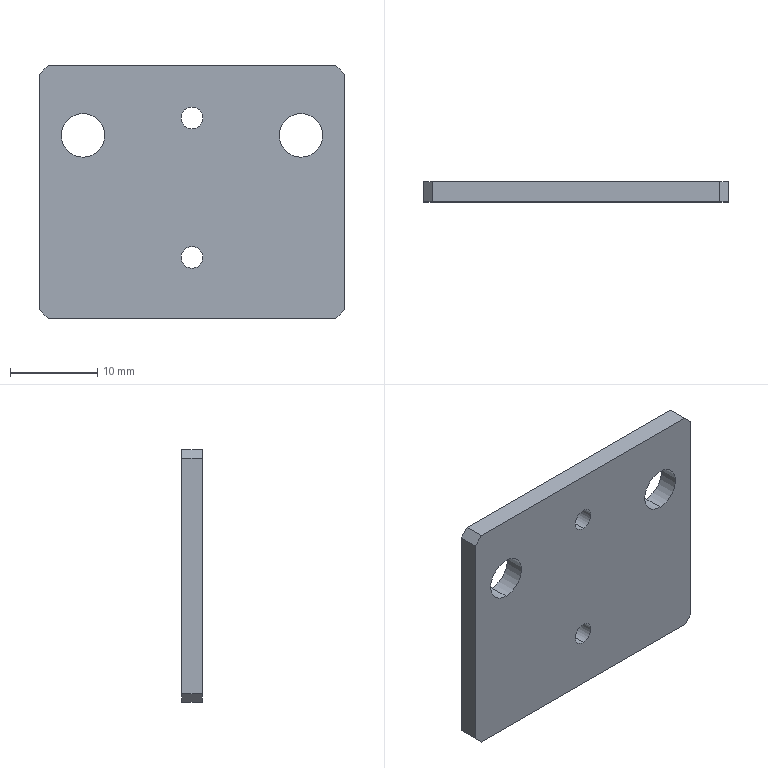Part | STEP file | 1105WWASensor BKT | 1 solid | 18 faces | box 35 x 2.3 x 29 mm | volume 2217 mm3 | plane 10 | cylinder 8 | commonest cylinder face diameters 2.5 x4 5 x4
STEP:
#1=CARTESIAN_POINT('',(-12.5,0.,9.));
#2=VERTEX_POINT('',#1);
#3=CARTESIAN_POINT('',(-12.5,0.,4.));
#4=VERTEX_POINT('',#3);
#5=CARTESIAN_POINT('',(-12.5,0.,6.5));
#6=DIRECTION('',(0.,-1.,0.));
#7=DIRECTION('',(0.,0.,-1.));
#8=AXIS2_PLACEMENT_3D('',#5,#6,#7);
#9=CIRCLE('',#8,2.5);
#10=EDGE_CURVE('',#2,#4,#9,.T.);
#11=ORIENTED_EDGE('',*,*,#10,.T.);
#12=CARTESIAN_POINT('',(-12.5,2.3,4.));
#13=VERTEX_POINT('',#12);
#14=CARTESIAN_POINT('',(-12.5,2.3,4.));
#15=DIRECTION('',(0.,1.,0.));
#16=VECTOR('',#15,1000.);
#17=LINE('',#14,#16);
#18=EDGE_CURVE('',#4,#13,#17,.T.);
#19=ORIENTED_EDGE('',*,*,#18,.T.);
#20=CARTESIAN_POINT('',(-12.5,2.3,9.));
#21=VERTEX_POINT('',#20);
#22=CARTESIAN_POINT('',(-12.5,2.3,6.5));
#23=DIRECTION('',(0.,1.,0.));
#24=DIRECTION('',(0.,0.,1.));
#25=AXIS2_PLACEMENT_3D('',#22,#23,#24);
#26=CIRCLE('',#25,2.5);
#27=EDGE_CURVE('',#13,#21,#26,.T.);
#28=ORIENTED_EDGE('',*,*,#27,.T.);
#29=CARTESIAN_POINT('',(-12.5,2.3,9.));
#30=DIRECTION('',(0.,1.,0.));
#31=VECTOR('',#30,1000.);
#32=LINE('',#29,#31);
#33=EDGE_CURVE('',#2,#21,#32,.T.);
#34=ORIENTED_EDGE('',*,*,#33,.F.);
#35=EDGE_LOOP('',(#11,#19,#28,#34));
#36=FACE_OUTER_BOUND('',#35,.T.);
#37=CARTESIAN_POINT('',(-12.5,2.3,6.5));
#38=DIRECTION('',(0.,1.,0.));
#39=DIRECTION('',(0.,0.,1.));
#40=AXIS2_PLACEMENT_3D('',#37,#38,#39);
#41=CYLINDRICAL_SURFACE('',#40,2.5);
#42=ADVANCED_FACE('',(#36),#41,.F.);
#43=CARTESIAN_POINT('',(12.5,0.,9.));
#44=VERTEX_POINT('',#43);
#45=CARTESIAN_POINT('',(12.5,0.,4.));
#46=VERTEX_POINT('',#45);
#47=CARTESIAN_POINT('',(12.5,0.,6.5));
#48=DIRECTION('',(0.,-1.,0.));
#49=DIRECTION('',(0.,0.,-1.));
#50=AXIS2_PLACEMENT_3D('',#47,#48,#49);
#51=CIRCLE('',#50,2.5);
#52=EDGE_CURVE('',#44,#46,#51,.T.);
#53=ORIENTED_EDGE('',*,*,#52,.T.);
#54=CARTESIAN_POINT('',(12.5,2.3,4.));
#55=VERTEX_POINT('',#54);
#56=CARTESIAN_POINT('',(12.5,2.3,4.));
#57=DIRECTION('',(0.,1.,0.));
#58=VECTOR('',#57,1000.);
#59=LINE('',#56,#58);
#60=EDGE_CURVE('',#46,#55,#59,.T.);
#61=ORIENTED_EDGE('',*,*,#60,.T.);
#62=CARTESIAN_POINT('',(12.5,2.3,9.));
#63=VERTEX_POINT('',#62);
#64=CARTESIAN_POINT('',(12.5,2.3,6.5));
#65=DIRECTION('',(0.,1.,0.));
#66=DIRECTION('',(0.,0.,1.));
#67=AXIS2_PLACEMENT_3D('',#64,#65,#66);
#68=CIRCLE('',#67,2.5);
#69=EDGE_CURVE('',#55,#63,#68,.T.);
#70=ORIENTED_EDGE('',*,*,#69,.T.);
#71=CARTESIAN_POINT('',(12.5,2.3,9.));
#72=DIRECTION('',(0.,1.,0.));
#73=VECTOR('',#72,1000.);
#74=LINE('',#71,#73);
#75=EDGE_CURVE('',#44,#63,#74,.T.);
#76=ORIENTED_EDGE('',*,*,#75,.F.);
#77=EDGE_LOOP('',(#53,#61,#70,#76));
#78=FACE_OUTER_BOUND('',#77,.T.);
#79=CARTESIAN_POINT('',(12.5,2.3,6.5));
#80=DIRECTION('',(0.,1.,0.));
#81=DIRECTION('',(0.,0.,1.));
#82=AXIS2_PLACEMENT_3D('',#79,#80,#81);
#83=CYLINDRICAL_SURFACE('',#82,2.5);
#84=ADVANCED_FACE('',(#78),#83,.F.);
#85=CARTESIAN_POINT('',(0.,0.,9.75));
#86=VERTEX_POINT('',#85);
#87=CARTESIAN_POINT('',(0.,0.,7.25));
#88=VERTEX_POINT('',#87);
#89=CARTESIAN_POINT('',(0.,0.,8.5));
#90=DIRECTION('',(0.,-1.,0.));
#91=DIRECTION('',(0.,0.,-1.));
#92=AXIS2_PLACEMENT_3D('',#89,#90,#91);
#93=CIRCLE('',#92,1.25);
#94=EDGE_CURVE('',#86,#88,#93,.T.);
#95=ORIENTED_EDGE('',*,*,#94,.T.);
#96=CARTESIAN_POINT('',(0.,2.3,7.25));
#97=VERTEX_POINT('',#96);
#98=CARTESIAN_POINT('',(0.,2.3,7.25));
#99=DIRECTION('',(0.,1.,0.));
#100=VECTOR('',#99,1000.);
#101=LINE('',#98,#100);
#102=EDGE_CURVE('',#88,#97,#101,.T.);
#103=ORIENTED_EDGE('',*,*,#102,.T.);
#104=CARTESIAN_POINT('',(0.,2.3,9.75));
#105=VERTEX_POINT('',#104);
#106=CARTESIAN_POINT('',(0.,2.3,8.5));
#107=DIRECTION('',(0.,1.,0.));
#108=DIRECTION('',(0.,0.,1.));
#109=AXIS2_PLACEMENT_3D('',#106,#107,#108);
#110=CIRCLE('',#109,1.25);
#111=EDGE_CURVE('',#97,#105,#110,.T.);
#112=ORIENTED_EDGE('',*,*,#111,.T.);
#113=CARTESIAN_POINT('',(0.,2.3,9.75));
#114=DIRECTION('',(0.,1.,0.));
#115=VECTOR('',#114,1000.);
#116=LINE('',#113,#115);
#117=EDGE_CURVE('',#86,#105,#116,.T.);
#118=ORIENTED_EDGE('',*,*,#117,.F.);
#119=EDGE_LOOP('',(#95,#103,#112,#118));
#120=FACE_OUTER_BOUND('',#119,.T.);
#121=CARTESIAN_POINT('',(0.,2.3,8.5));
#122=DIRECTION('',(0.,1.,0.));
#123=DIRECTION('',(0.,0.,1.));
#124=AXIS2_PLACEMENT_3D('',#121,#122,#123);
#125=CYLINDRICAL_SURFACE('',#124,1.25);
#126=ADVANCED_FACE('',(#120),#125,.F.);
#127=CARTESIAN_POINT('',(0.,0.,-6.25));
#128=VERTEX_POINT('',#127);
#129=CARTESIAN_POINT('',(0.,0.,-8.75));
#130=VERTEX_POINT('',#129);
#131=CARTESIAN_POINT('',(0.,0.,-7.5));
#132=DIRECTION('',(0.,-1.,0.));
#133=DIRECTION('',(0.,0.,-1.));
#134=AXIS2_PLACEMENT_3D('',#131,#132,#133);
#135=CIRCLE('',#134,1.25);
#136=EDGE_CURVE('',#128,#130,#135,.T.);
#137=ORIENTED_EDGE('',*,*,#136,.T.);
#138=CARTESIAN_POINT('',(0.,2.3,-8.75));
#139=VERTEX_POINT('',#138);
#140=CARTESIAN_POINT('',(0.,2.3,-8.75));
#141=DIRECTION('',(0.,1.,0.));
#142=VECTOR('',#141,1000.);
#143=LINE('',#140,#142);
#144=EDGE_CURVE('',#130,#139,#143,.T.);
#145=ORIENTED_EDGE('',*,*,#144,.T.);
#146=CARTESIAN_POINT('',(0.,2.3,-6.25));
#147=VERTEX_POINT('',#146);
#148=CARTESIAN_POINT('',(0.,2.3,-7.5));
#149=DIRECTION('',(0.,1.,0.));
#150=DIRECTION('',(0.,0.,1.));
#151=AXIS2_PLACEMENT_3D('',#148,#149,#150);
#152=CIRCLE('',#151,1.25);
#153=EDGE_CURVE('',#139,#147,#152,.T.);
#154=ORIENTED_EDGE('',*,*,#153,.T.);
#155=CARTESIAN_POINT('',(0.,2.3,-6.25));
#156=DIRECTION('',(0.,1.,0.));
#157=VECTOR('',#156,1000.);
#158=LINE('',#155,#157);
#159=EDGE_CURVE('',#128,#147,#158,.T.);
#160=ORIENTED_EDGE('',*,*,#159,.F.);
#161=EDGE_LOOP('',(#137,#145,#154,#160));
#162=FACE_OUTER_BOUND('',#161,.T.);
#163=CARTESIAN_POINT('',(0.,2.3,-7.5));
#164=DIRECTION('',(0.,1.,0.));
#165=DIRECTION('',(0.,0.,1.));
#166=AXIS2_PLACEMENT_3D('',#163,#164,#165);
#167=CYLINDRICAL_SURFACE('',#166,1.25);
#168=ADVANCED_FACE('',(#162),#167,.F.);
#169=CARTESIAN_POINT('',(17.5,0.,13.5));
#170=VERTEX_POINT('',#169);
#171=CARTESIAN_POINT('',(17.5,0.,-13.5));
#172=VERTEX_POINT('',#171);
#173=CARTESIAN_POINT('',(17.5,0.,14.5));
#174=DIRECTION('',(0.,0.,-1.));
#175=VECTOR('',#174,1000.);
#176=LINE('',#173,#175);
#177=EDGE_CURVE('',#170,#172,#176,.T.);
#178=ORIENTED_EDGE('',*,*,#177,.T.);
#179=CARTESIAN_POINT('',(17.5,2.3,-13.5));
#180=VERTEX_POINT('',#179);
#181=CARTESIAN_POINT('',(17.5,2.3,-13.5));
#182=DIRECTION('',(0.,1.,0.));
#183=VECTOR('',#182,1000.);
#184=LINE('',#181,#183);
#185=EDGE_CURVE('',#172,#180,#184,.T.);
#186=ORIENTED_EDGE('',*,*,#185,.T.);
#187=CARTESIAN_POINT('',(17.5,2.3,13.5));
#188=VERTEX_POINT('',#187);
#189=CARTESIAN_POINT('',(17.5,2.3,14.5));
#190=DIRECTION('',(0.,0.,-1.));
#191=VECTOR('',#190,1000.);
#192=LINE('',#189,#191);
#193=EDGE_CURVE('',#188,#180,#192,.T.);
#194=ORIENTED_EDGE('',*,*,#193,.F.);
#195=CARTESIAN_POINT('',(17.5,2.3,13.5));
#196=DIRECTION('',(0.,-1.,0.));
#197=VECTOR('',#196,1000.);
#198=LINE('',#195,#197);
#199=EDGE_CURVE('',#188,#170,#198,.T.);
#200=ORIENTED_EDGE('',*,*,#199,.T.);
#201=EDGE_LOOP('',(#178,#186,#194,#200));
#202=FACE_OUTER_BOUND('',#201,.T.);
#203=CARTESIAN_POINT('',(17.5,2.3,14.5));
#204=DIRECTION('',(-1.,0.,0.));
#205=DIRECTION('',(0.,0.,1.));
#206=AXIS2_PLACEMENT_3D('',#203,#204,#205);
#207=PLANE('',#206);
#208=ADVANCED_FACE('',(#202),#207,.F.);
#209=CARTESIAN_POINT('',(16.5,2.3,-14.5));
#210=VERTEX_POINT('',#209);
#211=CARTESIAN_POINT('',(-16.5,2.3,-14.5));
#212=VERTEX_POINT('',#211);
#213=CARTESIAN_POINT('',(-17.5,2.3,-14.5));
#214=DIRECTION('',(-1.,0.,0.));
#215=VECTOR('',#214,1000.);
#216=LINE('',#213,#215);
#217=EDGE_CURVE('',#210,#212,#216,.T.);
#218=ORIENTED_EDGE('',*,*,#217,.F.);
#219=CARTESIAN_POINT('',(16.5,0.,-14.5));
#220=VERTEX_POINT('',#219);
#221=CARTESIAN_POINT('',(16.5,2.3,-14.5));
#222=DIRECTION('',(0.,-1.,0.));
#223=VECTOR('',#222,1000.);
#224=LINE('',#221,#223);
#225=EDGE_CURVE('',#210,#220,#224,.T.);
#226=ORIENTED_EDGE('',*,*,#225,.T.);
#227=CARTESIAN_POINT('',(-16.5,0.,-14.5));
#228=VERTEX_POINT('',#227);
#229=CARTESIAN_POINT('',(-17.5,0.,-14.5));
#230=DIRECTION('',(-1.,0.,0.));
#231=VECTOR('',#230,1000.);
#232=LINE('',#229,#231);
#233=EDGE_CURVE('',#220,#228,#232,.T.);
#234=ORIENTED_EDGE('',*,*,#233,.T.);
#235=CARTESIAN_POINT('',(-16.5,2.3,-14.5));
#236=DIRECTION('',(0.,1.,0.));
#237=VECTOR('',#236,1000.);
#238=LINE('',#235,#237);
#239=EDGE_CURVE('',#228,#212,#238,.T.);
#240=ORIENTED_EDGE('',*,*,#239,.T.);
#241=EDGE_LOOP('',(#218,#226,#234,#240));
#242=FACE_OUTER_BOUND('',#241,.T.);
#243=CARTESIAN_POINT('',(-17.5,2.3,-14.5));
#244=DIRECTION('',(0.,0.,1.));
#245=DIRECTION('',(1.,0.,0.));
#246=AXIS2_PLACEMENT_3D('',#243,#244,#245);
#247=PLANE('',#246);
#248=ADVANCED_FACE('',(#242),#247,.F.);
#249=CARTESIAN_POINT('',(-17.5,2.3,-13.5));
#250=VERTEX_POINT('',#249);
#251=CARTESIAN_POINT('',(-17.5,2.3,13.5));
#252=VERTEX_POINT('',#251);
#253=CARTESIAN_POINT('',(-17.5,2.3,14.5));
#254=DIRECTION('',(0.,0.,1.));
#255=VECTOR('',#254,1000.);
#256=LINE('',#253,#255);
#257=EDGE_CURVE('',#250,#252,#256,.T.);
#258=ORIENTED_EDGE('',*,*,#257,.F.);
#259=CARTESIAN_POINT('',(-17.5,0.,-13.5));
#260=VERTEX_POINT('',#259);
#261=CARTESIAN_POINT('',(-17.5,2.3,-13.5));
#262=DIRECTION('',(0.,-1.,0.));
#263=VECTOR('',#262,1000.);
#264=LINE('',#261,#263);
#265=EDGE_CURVE('',#250,#260,#264,.T.);
#266=ORIENTED_EDGE('',*,*,#265,.T.);
#267=CARTESIAN_POINT('',(-17.5,0.,13.5));
#268=VERTEX_POINT('',#267);
#269=CARTESIAN_POINT('',(-17.5,0.,14.5));
#270=DIRECTION('',(0.,0.,1.));
#271=VECTOR('',#270,1000.);
#272=LINE('',#269,#271);
#273=EDGE_CURVE('',#260,#268,#272,.T.);
#274=ORIENTED_EDGE('',*,*,#273,.T.);
#275=CARTESIAN_POINT('',(-17.5,2.3,13.5));
#276=DIRECTION('',(0.,1.,0.));
#277=VECTOR('',#276,1000.);
#278=LINE('',#275,#277);
#279=EDGE_CURVE('',#268,#252,#278,.T.);
#280=ORIENTED_EDGE('',*,*,#279,.T.);
#281=EDGE_LOOP('',(#258,#266,#274,#280));
#282=FACE_OUTER_BOUND('',#281,.T.);
#283=CARTESIAN_POINT('',(-17.5,2.3,14.5));
#284=DIRECTION('',(1.,0.,0.));
#285=DIRECTION('',(0.,0.,-1.));
#286=AXIS2_PLACEMENT_3D('',#283,#284,#285);
#287=PLANE('',#286);
#288=ADVANCED_FACE('',(#282),#287,.F.);
#289=CARTESIAN_POINT('',(-16.5,0.,14.5));
#290=VERTEX_POINT('',#289);
#291=CARTESIAN_POINT('',(16.5,0.,14.5));
#292=VERTEX_POINT('',#291);
#293=CARTESIAN_POINT('',(-17.5,0.,14.5));
#294=DIRECTION('',(1.,0.,0.));
#295=VECTOR('',#294,1000.);
#296=LINE('',#293,#295);
#297=EDGE_CURVE('',#290,#292,#296,.T.);
#298=ORIENTED_EDGE('',*,*,#297,.T.);
#299=CARTESIAN_POINT('',(16.5,2.3,14.5));
#300=VERTEX_POINT('',#299);
#301=CARTESIAN_POINT('',(16.5,2.3,14.5));
#302=DIRECTION('',(0.,1.,0.));
#303=VECTOR('',#302,1000.);
#304=LINE('',#301,#303);
#305=EDGE_CURVE('',#292,#300,#304,.T.);
#306=ORIENTED_EDGE('',*,*,#305,.T.);
#307=CARTESIAN_POINT('',(-16.5,2.3,14.5));
#308=VERTEX_POINT('',#307);
#309=CARTESIAN_POINT('',(-17.5,2.3,14.5));
#310=DIRECTION('',(1.,0.,0.));
#311=VECTOR('',#310,1000.);
#312=LINE('',#309,#311);
#313=EDGE_CURVE('',#308,#300,#312,.T.);
#314=ORIENTED_EDGE('',*,*,#313,.F.);
#315=CARTESIAN_POINT('',(-16.5,2.3,14.5));
#316=DIRECTION('',(0.,-1.,0.));
#317=VECTOR('',#316,1000.);
#318=LINE('',#315,#317);
#319=EDGE_CURVE('',#308,#290,#318,.T.);
#320=ORIENTED_EDGE('',*,*,#319,.T.);
#321=EDGE_LOOP('',(#298,#306,#314,#320));
#322=FACE_OUTER_BOUND('',#321,.T.);
#323=CARTESIAN_POINT('',(-17.5,2.3,14.5));
#324=DIRECTION('',(0.,0.,-1.));
#325=DIRECTION('',(-1.,0.,0.));
#326=AXIS2_PLACEMENT_3D('',#323,#324,#325);
#327=PLANE('',#326);
#328=ADVANCED_FACE('',(#322),#327,.F.);
#329=CARTESIAN_POINT('',(-12.5,2.3,6.5));
#330=DIRECTION('',(0.,1.,0.));
#331=DIRECTION('',(0.,0.,1.));
#332=AXIS2_PLACEMENT_3D('',#329,#330,#331);
#333=CIRCLE('',#332,2.5);
#334=EDGE_CURVE('',#21,#13,#333,.T.);
#335=ORIENTED_EDGE('',*,*,#334,.F.);
#336=ORIENTED_EDGE('',*,*,#27,.F.);
#337=EDGE_LOOP('',(#335,#336));
#338=FACE_BOUND('',#337,.T.);
#339=CARTESIAN_POINT('',(12.5,2.3,6.5));
#340=DIRECTION('',(0.,1.,0.));
#341=DIRECTION('',(0.,0.,1.));
#342=AXIS2_PLACEMENT_3D('',#339,#340,#341);
#343=CIRCLE('',#342,2.5);
#344=EDGE_CURVE('',#63,#55,#343,.T.);
#345=ORIENTED_EDGE('',*,*,#344,.F.);
#346=ORIENTED_EDGE('',*,*,#69,.F.);
#347=EDGE_LOOP('',(#345,#346));
#348=FACE_BOUND('',#347,.T.);
#349=CARTESIAN_POINT('',(0.,2.3,8.5));
#350=DIRECTION('',(0.,1.,0.));
#351=DIRECTION('',(0.,0.,1.));
#352=AXIS2_PLACEMENT_3D('',#349,#350,#351);
#353=CIRCLE('',#352,1.25);
#354=EDGE_CURVE('',#105,#97,#353,.T.);
#355=ORIENTED_EDGE('',*,*,#354,.F.);
#356=ORIENTED_EDGE('',*,*,#111,.F.);
#357=EDGE_LOOP('',(#355,#356));
#358=FACE_BOUND('',#357,.T.);
#359=CARTESIAN_POINT('',(0.,2.3,-7.5));
#360=DIRECTION('',(0.,1.,0.));
#361=DIRECTION('',(0.,0.,1.));
#362=AXIS2_PLACEMENT_3D('',#359,#360,#361);
#363=CIRCLE('',#362,1.25);
#364=EDGE_CURVE('',#147,#139,#363,.T.);
#365=ORIENTED_EDGE('',*,*,#364,.F.);
#366=ORIENTED_EDGE('',*,*,#153,.F.);
#367=EDGE_LOOP('',(#365,#366));
#368=FACE_BOUND('',#367,.T.);
#369=ORIENTED_EDGE('',*,*,#193,.T.);
#370=CARTESIAN_POINT('',(16.5,2.3,-14.5));
#371=DIRECTION('',(-0.7071,0.,-0.7071));
#372=VECTOR('',#371,1000.);
#373=LINE('',#370,#372);
#374=EDGE_CURVE('',#180,#210,#373,.T.);
#375=ORIENTED_EDGE('',*,*,#374,.T.);
#376=ORIENTED_EDGE('',*,*,#217,.T.);
#377=CARTESIAN_POINT('',(-17.5,2.3,-13.5));
#378=DIRECTION('',(-0.7071,0.,0.7071));
#379=VECTOR('',#378,1000.);
#380=LINE('',#377,#379);
#381=EDGE_CURVE('',#212,#250,#380,.T.);
#382=ORIENTED_EDGE('',*,*,#381,.T.);
#383=ORIENTED_EDGE('',*,*,#257,.T.);
#384=CARTESIAN_POINT('',(-16.5,2.3,14.5));
#385=DIRECTION('',(0.7071,0.,0.7071));
#386=VECTOR('',#385,1000.);
#387=LINE('',#384,#386);
#388=EDGE_CURVE('',#252,#308,#387,.T.);
#389=ORIENTED_EDGE('',*,*,#388,.T.);
#390=ORIENTED_EDGE('',*,*,#313,.T.);
#391=CARTESIAN_POINT('',(17.5,2.3,13.5));
#392=DIRECTION('',(0.7071,0.,-0.7071));
#393=VECTOR('',#392,1000.);
#394=LINE('',#391,#393);
#395=EDGE_CURVE('',#300,#188,#394,.T.);
#396=ORIENTED_EDGE('',*,*,#395,.T.);
#397=EDGE_LOOP('',(#369,#375,#376,#382,#383,#389,#390,#396));
#398=FACE_OUTER_BOUND('',#397,.T.);
#399=CARTESIAN_POINT('',(17.5,2.3,-14.5));
#400=DIRECTION('',(0.,-1.,0.));
#401=DIRECTION('',(0.,0.,-1.));
#402=AXIS2_PLACEMENT_3D('',#399,#400,#401);
#403=PLANE('',#402);
#404=ADVANCED_FACE('',(#338,#348,#358,#368,#398),#403,.F.);
#405=ORIENTED_EDGE('',*,*,#10,.F.);
#406=CARTESIAN_POINT('',(-12.5,0.,6.5));
#407=DIRECTION('',(0.,-1.,0.));
#408=DIRECTION('',(0.,0.,-1.));
#409=AXIS2_PLACEMENT_3D('',#406,#407,#408);
#410=CIRCLE('',#409,2.5);
#411=EDGE_CURVE('',#4,#2,#410,.T.);
#412=ORIENTED_EDGE('',*,*,#411,.F.);
#413=EDGE_LOOP('',(#405,#412));
#414=FACE_BOUND('',#413,.T.);
#415=ORIENTED_EDGE('',*,*,#52,.F.);
#416=CARTESIAN_POINT('',(12.5,0.,6.5));
#417=DIRECTION('',(0.,-1.,0.));
#418=DIRECTION('',(0.,0.,-1.));
#419=AXIS2_PLACEMENT_3D('',#416,#417,#418);
#420=CIRCLE('',#419,2.5);
#421=EDGE_CURVE('',#46,#44,#420,.T.);
#422=ORIENTED_EDGE('',*,*,#421,.F.);
#423=EDGE_LOOP('',(#415,#422));
#424=FACE_BOUND('',#423,.T.);
#425=ORIENTED_EDGE('',*,*,#94,.F.);
#426=CARTESIAN_POINT('',(0.,0.,8.5));
#427=DIRECTION('',(0.,-1.,0.));
#428=DIRECTION('',(0.,0.,-1.));
#429=AXIS2_PLACEMENT_3D('',#426,#427,#428);
#430=CIRCLE('',#429,1.25);
#431=EDGE_CURVE('',#88,#86,#430,.T.);
#432=ORIENTED_EDGE('',*,*,#431,.F.);
#433=EDGE_LOOP('',(#425,#432));
#434=FACE_BOUND('',#433,.T.);
#435=ORIENTED_EDGE('',*,*,#136,.F.);
#436=CARTESIAN_POINT('',(0.,0.,-7.5));
#437=DIRECTION('',(0.,-1.,0.));
#438=DIRECTION('',(0.,0.,-1.));
#439=AXIS2_PLACEMENT_3D('',#436,#437,#438);
#440=CIRCLE('',#439,1.25);
#441=EDGE_CURVE('',#130,#128,#440,.T.);
#442=ORIENTED_EDGE('',*,*,#441,.F.);
#443=EDGE_LOOP('',(#435,#442));
#444=FACE_BOUND('',#443,.T.);
#445=ORIENTED_EDGE('',*,*,#233,.F.);
#446=CARTESIAN_POINT('',(17.,0.,-14.));
#447=DIRECTION('',(0.7071,0.,0.7071));
#448=VECTOR('',#447,1000.);
#449=LINE('',#446,#448);
#450=EDGE_CURVE('',#220,#172,#449,.T.);
#451=ORIENTED_EDGE('',*,*,#450,.T.);
#452=ORIENTED_EDGE('',*,*,#177,.F.);
#453=CARTESIAN_POINT('',(31.5,0.,-0.5));
#454=DIRECTION('',(-0.7071,0.,0.7071));
#455=VECTOR('',#454,1000.);
#456=LINE('',#453,#455);
#457=EDGE_CURVE('',#170,#292,#456,.T.);
#458=ORIENTED_EDGE('',*,*,#457,.T.);
#459=ORIENTED_EDGE('',*,*,#297,.F.);
#460=CARTESIAN_POINT('',(-14.,0.,17.));
#461=DIRECTION('',(-0.7071,0.,-0.7071));
#462=VECTOR('',#461,1000.);
#463=LINE('',#460,#462);
#464=EDGE_CURVE('',#290,#268,#463,.T.);
#465=ORIENTED_EDGE('',*,*,#464,.T.);
#466=ORIENTED_EDGE('',*,*,#273,.F.);
#467=CARTESIAN_POINT('',(0.5,0.,-31.5));
#468=DIRECTION('',(0.7071,0.,-0.7071));
#469=VECTOR('',#468,1000.);
#470=LINE('',#467,#469);
#471=EDGE_CURVE('',#260,#228,#470,.T.);
#472=ORIENTED_EDGE('',*,*,#471,.T.);
#473=EDGE_LOOP('',(#445,#451,#452,#458,#459,#465,#466,#472));
#474=FACE_OUTER_BOUND('',#473,.T.);
#475=CARTESIAN_POINT('',(17.5,0.,-14.5));
#476=DIRECTION('',(0.,-1.,0.));
#477=DIRECTION('',(0.,0.,-1.));
#478=AXIS2_PLACEMENT_3D('',#475,#476,#477);
#479=PLANE('',#478);
#480=ADVANCED_FACE('',(#414,#424,#434,#444,#474),#479,.T.);
#481=ORIENTED_EDGE('',*,*,#144,.F.);
#482=ORIENTED_EDGE('',*,*,#441,.T.);
#483=ORIENTED_EDGE('',*,*,#159,.T.);
#484=ORIENTED_EDGE('',*,*,#364,.T.);
#485=EDGE_LOOP('',(#481,#482,#483,#484));
#486=FACE_OUTER_BOUND('',#485,.T.);
#487=CARTESIAN_POINT('',(0.,2.3,-7.5));
#488=DIRECTION('',(0.,1.,0.));
#489=DIRECTION('',(0.,0.,1.));
#490=AXIS2_PLACEMENT_3D('',#487,#488,#489);
#491=CYLINDRICAL_SURFACE('',#490,1.25);
#492=ADVANCED_FACE('',(#486),#491,.F.);
#493=ORIENTED_EDGE('',*,*,#102,.F.);
#494=ORIENTED_EDGE('',*,*,#431,.T.);
#495=ORIENTED_EDGE('',*,*,#117,.T.);
#496=ORIENTED_EDGE('',*,*,#354,.T.);
#497=EDGE_LOOP('',(#493,#494,#495,#496));
#498=FACE_OUTER_BOUND('',#497,.T.);
#499=CARTESIAN_POINT('',(0.,2.3,8.5));
#500=DIRECTION('',(0.,1.,0.));
#501=DIRECTION('',(0.,0.,1.));
#502=AXIS2_PLACEMENT_3D('',#499,#500,#501);
#503=CYLINDRICAL_SURFACE('',#502,1.25);
#504=ADVANCED_FACE('',(#498),#503,.F.);
#505=ORIENTED_EDGE('',*,*,#60,.F.);
#506=ORIENTED_EDGE('',*,*,#421,.T.);
#507=ORIENTED_EDGE('',*,*,#75,.T.);
#508=ORIENTED_EDGE('',*,*,#344,.T.);
#509=EDGE_LOOP('',(#505,#506,#507,#508));
#510=FACE_OUTER_BOUND('',#509,.T.);
#511=CARTESIAN_POINT('',(12.5,2.3,6.5));
#512=DIRECTION('',(0.,1.,0.));
#513=DIRECTION('',(0.,0.,1.));
#514=AXIS2_PLACEMENT_3D('',#511,#512,#513);
#515=CYLINDRICAL_SURFACE('',#514,2.5);
#516=ADVANCED_FACE('',(#510),#515,.F.);
#517=ORIENTED_EDGE('',*,*,#18,.F.);
#518=ORIENTED_EDGE('',*,*,#411,.T.);
#519=ORIENTED_EDGE('',*,*,#33,.T.);
#520=ORIENTED_EDGE('',*,*,#334,.T.);
#521=EDGE_LOOP('',(#517,#518,#519,#520));
#522=FACE_OUTER_BOUND('',#521,.T.);
#523=CARTESIAN_POINT('',(-12.5,2.3,6.5));
#524=DIRECTION('',(0.,1.,0.));
#525=DIRECTION('',(0.,0.,1.));
#526=AXIS2_PLACEMENT_3D('',#523,#524,#525);
#527=CYLINDRICAL_SURFACE('',#526,2.5);
#528=ADVANCED_FACE('',(#522),#527,.F.);
#529=ORIENTED_EDGE('',*,*,#374,.F.);
#530=ORIENTED_EDGE('',*,*,#185,.F.);
#531=ORIENTED_EDGE('',*,*,#450,.F.);
#532=ORIENTED_EDGE('',*,*,#225,.F.);
#533=EDGE_LOOP('',(#529,#530,#531,#532));
#534=FACE_OUTER_BOUND('',#533,.T.);
#535=CARTESIAN_POINT('',(16.5,2.3,-14.5));
#536=DIRECTION('',(-0.7071,0.,0.7071));
#537=DIRECTION('',(0.7071,0.,0.7071));
#538=AXIS2_PLACEMENT_3D('',#535,#536,#537);
#539=PLANE('',#538);
#540=ADVANCED_FACE('',(#534),#539,.F.);
#541=ORIENTED_EDGE('',*,*,#381,.F.);
#542=ORIENTED_EDGE('',*,*,#239,.F.);
#543=ORIENTED_EDGE('',*,*,#471,.F.);
#544=ORIENTED_EDGE('',*,*,#265,.F.);
#545=EDGE_LOOP('',(#541,#542,#543,#544));
#546=FACE_OUTER_BOUND('',#545,.T.);
#547=CARTESIAN_POINT('',(-17.5,2.3,-13.5));
#548=DIRECTION('',(0.7071,0.,0.7071));
#549=DIRECTION('',(0.7071,0.,-0.7071));
#550=AXIS2_PLACEMENT_3D('',#547,#548,#549);
#551=PLANE('',#550);
#552=ADVANCED_FACE('',(#546),#551,.F.);
#553=ORIENTED_EDGE('',*,*,#395,.F.);
#554=ORIENTED_EDGE('',*,*,#305,.F.);
#555=ORIENTED_EDGE('',*,*,#457,.F.);
#556=ORIENTED_EDGE('',*,*,#199,.F.);
#557=EDGE_LOOP('',(#553,#554,#555,#556));
#558=FACE_OUTER_BOUND('',#557,.T.);
#559=CARTESIAN_POINT('',(17.5,2.3,13.5));
#560=DIRECTION('',(-0.7071,0.,-0.7071));
#561=DIRECTION('',(-0.7071,0.,0.7071));
#562=AXIS2_PLACEMENT_3D('',#559,#560,#561);
#563=PLANE('',#562);
#564=ADVANCED_FACE('',(#558),#563,.F.);
#565=ORIENTED_EDGE('',*,*,#388,.F.);
#566=ORIENTED_EDGE('',*,*,#279,.F.);
#567=ORIENTED_EDGE('',*,*,#464,.F.);
#568=ORIENTED_EDGE('',*,*,#319,.F.);
#569=EDGE_LOOP('',(#565,#566,#567,#568));
#570=FACE_OUTER_BOUND('',#569,.T.);
#571=CARTESIAN_POINT('',(-16.5,2.3,14.5));
#572=DIRECTION('',(0.7071,0.,-0.7071));
#573=DIRECTION('',(-0.7071,0.,-0.7071));
#574=AXIS2_PLACEMENT_3D('',#571,#572,#573);
#575=PLANE('',#574);
#576=ADVANCED_FACE('',(#570),#575,.F.);
#577=CLOSED_SHELL('',(#42,#84,#126,#168,#208,#248,#288,#328,#404,#480,#492,#504,#516,#528,#540,#552,#564,#576));
#578=MANIFOLD_SOLID_BREP('',#577);
#579=CARTESIAN_POINT('',(0.,0.,0.));
#580=DIRECTION('',(0.,0.,1.));
#581=DIRECTION('',(1.,0.,0.));
#582=AXIS2_PLACEMENT_3D('',#579,#580,#581);
#583=(LENGTH_UNIT()NAMED_UNIT(*)SI_UNIT(.MILLI.,.METRE.));
#584=UNCERTAINTY_MEASURE_WITH_UNIT(LENGTH_MEASURE(0.00001),#583,'','');
#585=(NAMED_UNIT(*)PLANE_ANGLE_UNIT()SI_UNIT($,.RADIAN.));
#586=(NAMED_UNIT(*)SI_UNIT($,.STERADIAN.)SOLID_ANGLE_UNIT());
#587=(GEOMETRIC_REPRESENTATION_CONTEXT(3)GLOBAL_UNCERTAINTY_ASSIGNED_CONTEXT((#584))GLOBAL_UNIT_ASSIGNED_CONTEXT((#583,#585,#586))REPRESENTATION_CONTEXT('',''));
#588=ADVANCED_BREP_SHAPE_REPRESENTATION('',(#578,#582),#587);